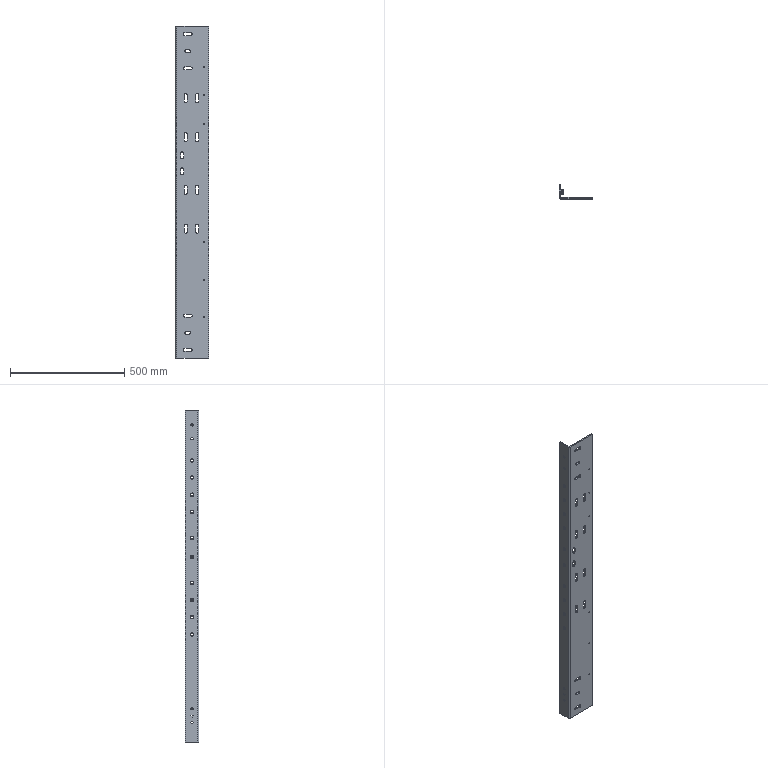Part | SolidWorks | 11 solids | 411 faces | box 145 x 60 x 1450 mm | volume 1682863 mm3 | plane 207 | cylinder 144 | cone 60 | commonest cylinder face diameters 14 x24 10.647 x20 14.75 x20 15 x20 15.07 x20 13 x14